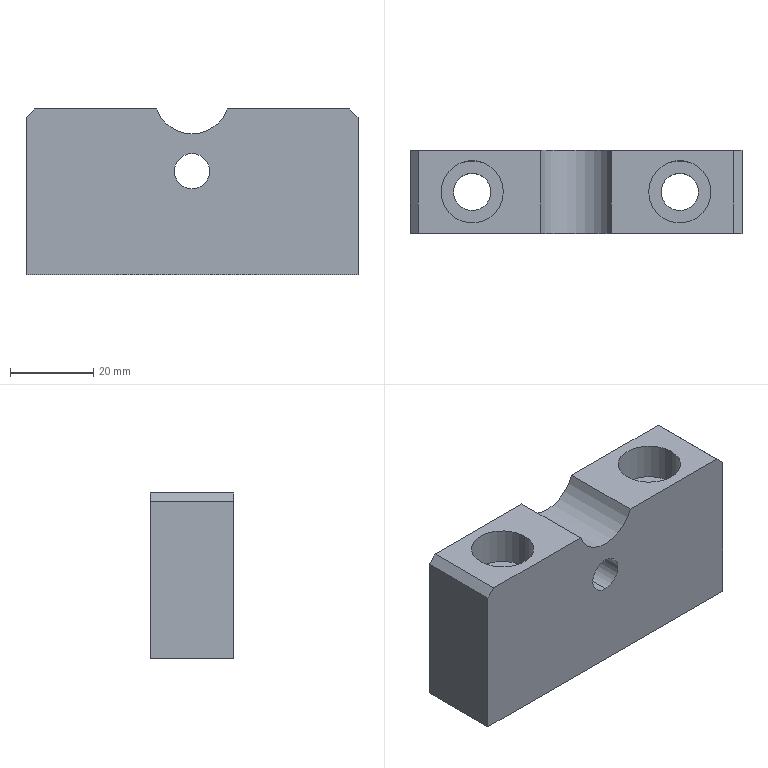Part | STEP file | fBY02F02M-00-10A | 1 solid | 22 faces | box 80 x 20 x 40 mm | volume 54175 mm3 | cylinder 11 | plane 11 | commonest cylinder face diameters 9 x4 15 x4 8.5 x2 18 x1